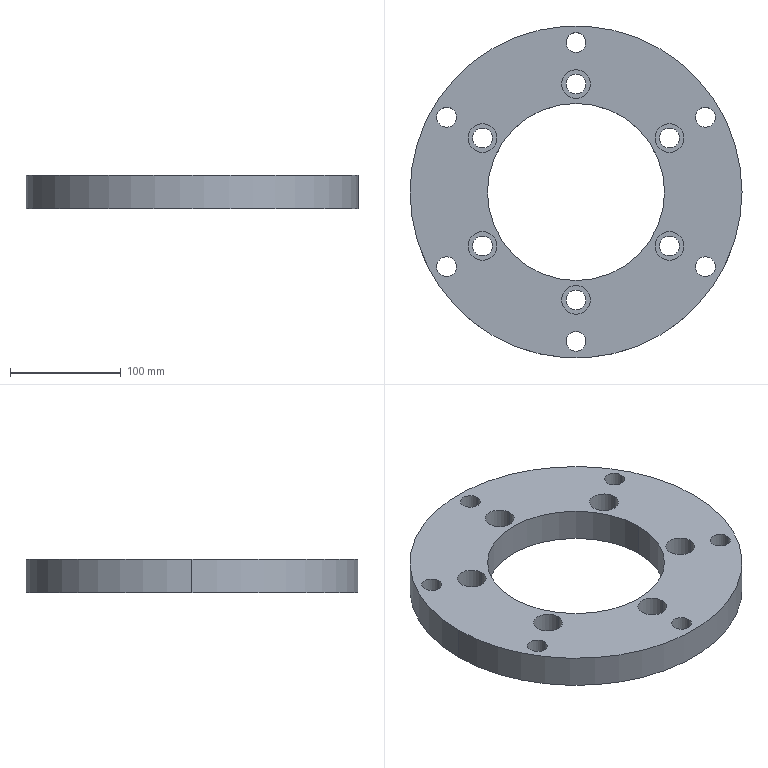Part | SolidWorks | features ICE 3, Extrusion 1 | 1 solid | 48 faces | box 300 x 300 x 30 mm | volume 1392605 mm3 | cylinder 40 | plane 8 | commonest cylinder face diameters 18 x24 26 x12 160 x2 300 x2
STEP:
#1=CARTESIAN_POINT('',(71.437,48.75,10.));
#2=VERTEX_POINT('',#1);
#3=CARTESIAN_POINT('',(97.437,48.75,10.));
#4=VERTEX_POINT('',#3);
#5=CARTESIAN_POINT('',(84.437,48.75,10.));
#6=DIRECTION('',(0.,0.,1.));
#7=DIRECTION('',(1.,0.,0.));
#8=AXIS2_PLACEMENT_3D('',#5,#6,#7);
#9=CIRCLE('',#8,13.);
#10=EDGE_CURVE('',#2,#4,#9,.T.);
#11=ORIENTED_EDGE('',*,*,#10,.F.);
#12=CARTESIAN_POINT('',(71.437,48.75,30.));
#13=VERTEX_POINT('',#12);
#14=CARTESIAN_POINT('',(71.437,48.75,10.));
#15=DIRECTION('',(0.,0.,1.));
#16=VECTOR('',#15,1000.);
#17=LINE('',#14,#16);
#18=EDGE_CURVE('',#2,#13,#17,.T.);
#19=ORIENTED_EDGE('',*,*,#18,.T.);
#20=CARTESIAN_POINT('',(97.437,48.75,30.));
#21=VERTEX_POINT('',#20);
#22=CARTESIAN_POINT('',(84.437,48.75,30.));
#23=DIRECTION('',(0.,0.,1.));
#24=DIRECTION('',(1.,0.,0.));
#25=AXIS2_PLACEMENT_3D('',#22,#23,#24);
#26=CIRCLE('',#25,13.);
#27=EDGE_CURVE('',#13,#21,#26,.T.);
#28=ORIENTED_EDGE('',*,*,#27,.T.);
#29=CARTESIAN_POINT('',(97.437,48.75,10.));
#30=DIRECTION('',(0.,0.,1.));
#31=VECTOR('',#30,1000.);
#32=LINE('',#29,#31);
#33=EDGE_CURVE('',#4,#21,#32,.T.);
#34=ORIENTED_EDGE('',*,*,#33,.F.);
#35=EDGE_LOOP('',(#11,#19,#28,#34));
#36=FACE_OUTER_BOUND('',#35,.T.);
#37=CARTESIAN_POINT('',(84.437,48.75,10.));
#38=DIRECTION('',(0.,0.,1.));
#39=DIRECTION('',(1.,0.,0.));
#40=AXIS2_PLACEMENT_3D('',#37,#38,#39);
#41=CYLINDRICAL_SURFACE('',#40,13.);
#42=ADVANCED_FACE('',(#36),#41,.F.);
#43=CARTESIAN_POINT('',(71.437,-48.75,10.));
#44=VERTEX_POINT('',#43);
#45=CARTESIAN_POINT('',(97.437,-48.75,10.));
#46=VERTEX_POINT('',#45);
#47=CARTESIAN_POINT('',(84.437,-48.75,10.));
#48=DIRECTION('',(0.,0.,1.));
#49=DIRECTION('',(1.,0.,0.));
#50=AXIS2_PLACEMENT_3D('',#47,#48,#49);
#51=CIRCLE('',#50,13.);
#52=EDGE_CURVE('',#44,#46,#51,.T.);
#53=ORIENTED_EDGE('',*,*,#52,.F.);
#54=CARTESIAN_POINT('',(71.437,-48.75,30.));
#55=VERTEX_POINT('',#54);
#56=CARTESIAN_POINT('',(71.437,-48.75,10.));
#57=DIRECTION('',(0.,0.,1.));
#58=VECTOR('',#57,1000.);
#59=LINE('',#56,#58);
#60=EDGE_CURVE('',#44,#55,#59,.T.);
#61=ORIENTED_EDGE('',*,*,#60,.T.);
#62=CARTESIAN_POINT('',(97.437,-48.75,30.));
#63=VERTEX_POINT('',#62);
#64=CARTESIAN_POINT('',(84.437,-48.75,30.));
#65=DIRECTION('',(0.,0.,1.));
#66=DIRECTION('',(1.,0.,0.));
#67=AXIS2_PLACEMENT_3D('',#64,#65,#66);
#68=CIRCLE('',#67,13.);
#69=EDGE_CURVE('',#55,#63,#68,.T.);
#70=ORIENTED_EDGE('',*,*,#69,.T.);
#71=CARTESIAN_POINT('',(97.437,-48.75,10.));
#72=DIRECTION('',(0.,0.,1.));
#73=VECTOR('',#72,1000.);
#74=LINE('',#71,#73);
#75=EDGE_CURVE('',#46,#63,#74,.T.);
#76=ORIENTED_EDGE('',*,*,#75,.F.);
#77=EDGE_LOOP('',(#53,#61,#70,#76));
#78=FACE_OUTER_BOUND('',#77,.T.);
#79=CARTESIAN_POINT('',(84.437,-48.75,10.));
#80=DIRECTION('',(0.,0.,1.));
#81=DIRECTION('',(1.,0.,0.));
#82=AXIS2_PLACEMENT_3D('',#79,#80,#81);
#83=CYLINDRICAL_SURFACE('',#82,13.);
#84=ADVANCED_FACE('',(#78),#83,.F.);
#85=CARTESIAN_POINT('',(-13.,-97.5,10.));
#86=VERTEX_POINT('',#85);
#87=CARTESIAN_POINT('',(13.,-97.5,10.));
#88=VERTEX_POINT('',#87);
#89=CARTESIAN_POINT('',(0.,-97.5,10.));
#90=DIRECTION('',(0.,0.,1.));
#91=DIRECTION('',(1.,0.,0.));
#92=AXIS2_PLACEMENT_3D('',#89,#90,#91);
#93=CIRCLE('',#92,13.);
#94=EDGE_CURVE('',#86,#88,#93,.T.);
#95=ORIENTED_EDGE('',*,*,#94,.F.);
#96=CARTESIAN_POINT('',(-13.,-97.5,30.));
#97=VERTEX_POINT('',#96);
#98=CARTESIAN_POINT('',(-13.,-97.5,10.));
#99=DIRECTION('',(0.,0.,1.));
#100=VECTOR('',#99,1000.);
#101=LINE('',#98,#100);
#102=EDGE_CURVE('',#86,#97,#101,.T.);
#103=ORIENTED_EDGE('',*,*,#102,.T.);
#104=CARTESIAN_POINT('',(13.,-97.5,30.));
#105=VERTEX_POINT('',#104);
#106=CARTESIAN_POINT('',(0.,-97.5,30.));
#107=DIRECTION('',(0.,0.,1.));
#108=DIRECTION('',(1.,0.,0.));
#109=AXIS2_PLACEMENT_3D('',#106,#107,#108);
#110=CIRCLE('',#109,13.);
#111=EDGE_CURVE('',#97,#105,#110,.T.);
#112=ORIENTED_EDGE('',*,*,#111,.T.);
#113=CARTESIAN_POINT('',(13.,-97.5,10.));
#114=DIRECTION('',(0.,0.,1.));
#115=VECTOR('',#114,1000.);
#116=LINE('',#113,#115);
#117=EDGE_CURVE('',#88,#105,#116,.T.);
#118=ORIENTED_EDGE('',*,*,#117,.F.);
#119=EDGE_LOOP('',(#95,#103,#112,#118));
#120=FACE_OUTER_BOUND('',#119,.T.);
#121=CARTESIAN_POINT('',(0.,-97.5,10.));
#122=DIRECTION('',(0.,0.,1.));
#123=DIRECTION('',(1.,0.,0.));
#124=AXIS2_PLACEMENT_3D('',#121,#122,#123);
#125=CYLINDRICAL_SURFACE('',#124,13.);
#126=ADVANCED_FACE('',(#120),#125,.F.);
#127=CARTESIAN_POINT('',(-97.437,-48.75,10.));
#128=VERTEX_POINT('',#127);
#129=CARTESIAN_POINT('',(-71.437,-48.75,10.));
#130=VERTEX_POINT('',#129);
#131=CARTESIAN_POINT('',(-84.437,-48.75,10.));
#132=DIRECTION('',(0.,0.,1.));
#133=DIRECTION('',(1.,0.,0.));
#134=AXIS2_PLACEMENT_3D('',#131,#132,#133);
#135=CIRCLE('',#134,13.);
#136=EDGE_CURVE('',#128,#130,#135,.T.);
#137=ORIENTED_EDGE('',*,*,#136,.F.);
#138=CARTESIAN_POINT('',(-97.437,-48.75,30.));
#139=VERTEX_POINT('',#138);
#140=CARTESIAN_POINT('',(-97.437,-48.75,10.));
#141=DIRECTION('',(0.,0.,1.));
#142=VECTOR('',#141,1000.);
#143=LINE('',#140,#142);
#144=EDGE_CURVE('',#128,#139,#143,.T.);
#145=ORIENTED_EDGE('',*,*,#144,.T.);
#146=CARTESIAN_POINT('',(-71.437,-48.75,30.));
#147=VERTEX_POINT('',#146);
#148=CARTESIAN_POINT('',(-84.437,-48.75,30.));
#149=DIRECTION('',(0.,0.,1.));
#150=DIRECTION('',(1.,0.,0.));
#151=AXIS2_PLACEMENT_3D('',#148,#149,#150);
#152=CIRCLE('',#151,13.);
#153=EDGE_CURVE('',#139,#147,#152,.T.);
#154=ORIENTED_EDGE('',*,*,#153,.T.);
#155=CARTESIAN_POINT('',(-71.437,-48.75,10.));
#156=DIRECTION('',(0.,0.,1.));
#157=VECTOR('',#156,1000.);
#158=LINE('',#155,#157);
#159=EDGE_CURVE('',#130,#147,#158,.T.);
#160=ORIENTED_EDGE('',*,*,#159,.F.);
#161=EDGE_LOOP('',(#137,#145,#154,#160));
#162=FACE_OUTER_BOUND('',#161,.T.);
#163=CARTESIAN_POINT('',(-84.437,-48.75,10.));
#164=DIRECTION('',(0.,0.,1.));
#165=DIRECTION('',(1.,0.,0.));
#166=AXIS2_PLACEMENT_3D('',#163,#164,#165);
#167=CYLINDRICAL_SURFACE('',#166,13.);
#168=ADVANCED_FACE('',(#162),#167,.F.);
#169=CARTESIAN_POINT('',(-97.437,48.75,10.));
#170=VERTEX_POINT('',#169);
#171=CARTESIAN_POINT('',(-71.437,48.75,10.));
#172=VERTEX_POINT('',#171);
#173=CARTESIAN_POINT('',(-84.437,48.75,10.));
#174=DIRECTION('',(0.,0.,1.));
#175=DIRECTION('',(1.,0.,0.));
#176=AXIS2_PLACEMENT_3D('',#173,#174,#175);
#177=CIRCLE('',#176,13.);
#178=EDGE_CURVE('',#170,#172,#177,.T.);
#179=ORIENTED_EDGE('',*,*,#178,.F.);
#180=CARTESIAN_POINT('',(-97.437,48.75,30.));
#181=VERTEX_POINT('',#180);
#182=CARTESIAN_POINT('',(-97.437,48.75,10.));
#183=DIRECTION('',(0.,0.,1.));
#184=VECTOR('',#183,1000.);
#185=LINE('',#182,#184);
#186=EDGE_CURVE('',#170,#181,#185,.T.);
#187=ORIENTED_EDGE('',*,*,#186,.T.);
#188=CARTESIAN_POINT('',(-71.437,48.75,30.));
#189=VERTEX_POINT('',#188);
#190=CARTESIAN_POINT('',(-84.437,48.75,30.));
#191=DIRECTION('',(0.,0.,1.));
#192=DIRECTION('',(1.,0.,0.));
#193=AXIS2_PLACEMENT_3D('',#190,#191,#192);
#194=CIRCLE('',#193,13.);
#195=EDGE_CURVE('',#181,#189,#194,.T.);
#196=ORIENTED_EDGE('',*,*,#195,.T.);
#197=CARTESIAN_POINT('',(-71.437,48.75,10.));
#198=DIRECTION('',(0.,0.,1.));
#199=VECTOR('',#198,1000.);
#200=LINE('',#197,#199);
#201=EDGE_CURVE('',#172,#189,#200,.T.);
#202=ORIENTED_EDGE('',*,*,#201,.F.);
#203=EDGE_LOOP('',(#179,#187,#196,#202));
#204=FACE_OUTER_BOUND('',#203,.T.);
#205=CARTESIAN_POINT('',(-84.437,48.75,10.));
#206=DIRECTION('',(0.,0.,1.));
#207=DIRECTION('',(1.,0.,0.));
#208=AXIS2_PLACEMENT_3D('',#205,#206,#207);
#209=CYLINDRICAL_SURFACE('',#208,13.);
#210=ADVANCED_FACE('',(#204),#209,.F.);
#211=CARTESIAN_POINT('',(-13.,97.5,10.));
#212=VERTEX_POINT('',#211);
#213=CARTESIAN_POINT('',(13.,97.5,10.));
#214=VERTEX_POINT('',#213);
#215=CARTESIAN_POINT('',(0.,97.5,10.));
#216=DIRECTION('',(0.,0.,1.));
#217=DIRECTION('',(1.,0.,0.));
#218=AXIS2_PLACEMENT_3D('',#215,#216,#217);
#219=CIRCLE('',#218,13.);
#220=EDGE_CURVE('',#212,#214,#219,.T.);
#221=ORIENTED_EDGE('',*,*,#220,.F.);
#222=CARTESIAN_POINT('',(-13.,97.5,30.));
#223=VERTEX_POINT('',#222);
#224=CARTESIAN_POINT('',(-13.,97.5,10.));
#225=DIRECTION('',(0.,0.,1.));
#226=VECTOR('',#225,1000.);
#227=LINE('',#224,#226);
#228=EDGE_CURVE('',#212,#223,#227,.T.);
#229=ORIENTED_EDGE('',*,*,#228,.T.);
#230=CARTESIAN_POINT('',(13.,97.5,30.));
#231=VERTEX_POINT('',#230);
#232=CARTESIAN_POINT('',(0.,97.5,30.));
#233=DIRECTION('',(0.,0.,1.));
#234=DIRECTION('',(1.,0.,0.));
#235=AXIS2_PLACEMENT_3D('',#232,#233,#234);
#236=CIRCLE('',#235,13.);
#237=EDGE_CURVE('',#223,#231,#236,.T.);
#238=ORIENTED_EDGE('',*,*,#237,.T.);
#239=CARTESIAN_POINT('',(13.,97.5,10.));
#240=DIRECTION('',(0.,0.,1.));
#241=VECTOR('',#240,1000.);
#242=LINE('',#239,#241);
#243=EDGE_CURVE('',#214,#231,#242,.T.);
#244=ORIENTED_EDGE('',*,*,#243,.F.);
#245=EDGE_LOOP('',(#221,#229,#238,#244));
#246=FACE_OUTER_BOUND('',#245,.T.);
#247=CARTESIAN_POINT('',(0.,97.5,10.));
#248=DIRECTION('',(0.,0.,1.));
#249=DIRECTION('',(1.,0.,0.));
#250=AXIS2_PLACEMENT_3D('',#247,#248,#249);
#251=CYLINDRICAL_SURFACE('',#250,13.);
#252=ADVANCED_FACE('',(#246),#251,.F.);
#253=CARTESIAN_POINT('',(-9.,135.,0.));
#254=VERTEX_POINT('',#253);
#255=CARTESIAN_POINT('',(9.,135.,0.));
#256=VERTEX_POINT('',#255);
#257=CARTESIAN_POINT('',(0.,135.,0.));
#258=DIRECTION('',(0.,0.,1.));
#259=DIRECTION('',(1.,0.,0.));
#260=AXIS2_PLACEMENT_3D('',#257,#258,#259);
#261=CIRCLE('',#260,9.);
#262=EDGE_CURVE('',#254,#256,#261,.T.);
#263=ORIENTED_EDGE('',*,*,#262,.F.);
#264=CARTESIAN_POINT('',(-9.,135.,30.));
#265=VERTEX_POINT('',#264);
#266=CARTESIAN_POINT('',(-9.,135.,0.));
#267=DIRECTION('',(0.,0.,1.));
#268=VECTOR('',#267,1000.);
#269=LINE('',#266,#268);
#270=EDGE_CURVE('',#254,#265,#269,.T.);
#271=ORIENTED_EDGE('',*,*,#270,.T.);
#272=CARTESIAN_POINT('',(9.,135.,30.));
#273=VERTEX_POINT('',#272);
#274=CARTESIAN_POINT('',(0.,135.,30.));
#275=DIRECTION('',(0.,0.,1.));
#276=DIRECTION('',(1.,0.,0.));
#277=AXIS2_PLACEMENT_3D('',#274,#275,#276);
#278=CIRCLE('',#277,9.);
#279=EDGE_CURVE('',#265,#273,#278,.T.);
#280=ORIENTED_EDGE('',*,*,#279,.T.);
#281=CARTESIAN_POINT('',(9.,135.,0.));
#282=DIRECTION('',(0.,0.,1.));
#283=VECTOR('',#282,1000.);
#284=LINE('',#281,#283);
#285=EDGE_CURVE('',#256,#273,#284,.T.);
#286=ORIENTED_EDGE('',*,*,#285,.F.);
#287=EDGE_LOOP('',(#263,#271,#280,#286));
#288=FACE_OUTER_BOUND('',#287,.T.);
#289=CARTESIAN_POINT('',(0.,135.,0.));
#290=DIRECTION('',(0.,0.,1.));
#291=DIRECTION('',(1.,0.,0.));
#292=AXIS2_PLACEMENT_3D('',#289,#290,#291);
#293=CYLINDRICAL_SURFACE('',#292,9.);
#294=ADVANCED_FACE('',(#288),#293,.F.);
#295=CARTESIAN_POINT('',(-125.913,67.5,0.));
#296=VERTEX_POINT('',#295);
#297=CARTESIAN_POINT('',(-107.913,67.5,0.));
#298=VERTEX_POINT('',#297);
#299=CARTESIAN_POINT('',(-116.913,67.5,0.));
#300=DIRECTION('',(0.,0.,1.));
#301=DIRECTION('',(1.,0.,0.));
#302=AXIS2_PLACEMENT_3D('',#299,#300,#301);
#303=CIRCLE('',#302,9.);
#304=EDGE_CURVE('',#296,#298,#303,.T.);
#305=ORIENTED_EDGE('',*,*,#304,.F.);
#306=CARTESIAN_POINT('',(-125.913,67.5,30.));
#307=VERTEX_POINT('',#306);
#308=CARTESIAN_POINT('',(-125.913,67.5,0.));
#309=DIRECTION('',(0.,0.,1.));
#310=VECTOR('',#309,1000.);
#311=LINE('',#308,#310);
#312=EDGE_CURVE('',#296,#307,#311,.T.);
#313=ORIENTED_EDGE('',*,*,#312,.T.);
#314=CARTESIAN_POINT('',(-107.913,67.5,30.));
#315=VERTEX_POINT('',#314);
#316=CARTESIAN_POINT('',(-116.913,67.5,30.));
#317=DIRECTION('',(0.,0.,1.));
#318=DIRECTION('',(1.,0.,0.));
#319=AXIS2_PLACEMENT_3D('',#316,#317,#318);
#320=CIRCLE('',#319,9.);
#321=EDGE_CURVE('',#307,#315,#320,.T.);
#322=ORIENTED_EDGE('',*,*,#321,.T.);
#323=CARTESIAN_POINT('',(-107.913,67.5,0.));
#324=DIRECTION('',(0.,0.,1.));
#325=VECTOR('',#324,1000.);
#326=LINE('',#323,#325);
#327=EDGE_CURVE('',#298,#315,#326,.T.);
#328=ORIENTED_EDGE('',*,*,#327,.F.);
#329=EDGE_LOOP('',(#305,#313,#322,#328));
#330=FACE_OUTER_BOUND('',#329,.T.);
#331=CARTESIAN_POINT('',(-116.913,67.5,0.));
#332=DIRECTION('',(0.,0.,1.));
#333=DIRECTION('',(1.,0.,0.));
#334=AXIS2_PLACEMENT_3D('',#331,#332,#333);
#335=CYLINDRICAL_SURFACE('',#334,9.);
#336=ADVANCED_FACE('',(#330),#335,.F.);
#337=CARTESIAN_POINT('',(-125.913,-67.5,0.));
#338=VERTEX_POINT('',#337);
#339=CARTESIAN_POINT('',(-107.913,-67.5,0.));
#340=VERTEX_POINT('',#339);
#341=CARTESIAN_POINT('',(-116.913,-67.5,0.));
#342=DIRECTION('',(0.,0.,1.));
#343=DIRECTION('',(1.,0.,0.));
#344=AXIS2_PLACEMENT_3D('',#341,#342,#343);
#345=CIRCLE('',#344,9.);
#346=EDGE_CURVE('',#338,#340,#345,.T.);
#347=ORIENTED_EDGE('',*,*,#346,.F.);
#348=CARTESIAN_POINT('',(-125.913,-67.5,30.));
#349=VERTEX_POINT('',#348);
#350=CARTESIAN_POINT('',(-125.913,-67.5,0.));
#351=DIRECTION('',(0.,0.,1.));
#352=VECTOR('',#351,1000.);
#353=LINE('',#350,#352);
#354=EDGE_CURVE('',#338,#349,#353,.T.);
#355=ORIENTED_EDGE('',*,*,#354,.T.);
#356=CARTESIAN_POINT('',(-107.913,-67.5,30.));
#357=VERTEX_POINT('',#356);
#358=CARTESIAN_POINT('',(-116.913,-67.5,30.));
#359=DIRECTION('',(0.,0.,1.));
#360=DIRECTION('',(1.,0.,0.));
#361=AXIS2_PLACEMENT_3D('',#358,#359,#360);
#362=CIRCLE('',#361,9.);
#363=EDGE_CURVE('',#349,#357,#362,.T.);
#364=ORIENTED_EDGE('',*,*,#363,.T.);
#365=CARTESIAN_POINT('',(-107.913,-67.5,0.));
#366=DIRECTION('',(0.,0.,1.));
#367=VECTOR('',#366,1000.);
#368=LINE('',#365,#367);
#369=EDGE_CURVE('',#340,#357,#368,.T.);
#370=ORIENTED_EDGE('',*,*,#369,.F.);
#371=EDGE_LOOP('',(#347,#355,#364,#370));
#372=FACE_OUTER_BOUND('',#371,.T.);
#373=CARTESIAN_POINT('',(-116.913,-67.5,0.));
#374=DIRECTION('',(0.,0.,1.));
#375=DIRECTION('',(1.,0.,0.));
#376=AXIS2_PLACEMENT_3D('',#373,#374,#375);
#377=CYLINDRICAL_SURFACE('',#376,9.);
#378=ADVANCED_FACE('',(#372),#377,.F.);
#379=CARTESIAN_POINT('',(-9.,-135.,0.));
#380=VERTEX_POINT('',#379);
#381=CARTESIAN_POINT('',(9.,-135.,0.));
#382=VERTEX_POINT('',#381);
#383=CARTESIAN_POINT('',(0.,-135.,0.));
#384=DIRECTION('',(0.,0.,1.));
#385=DIRECTION('',(1.,0.,0.));
#386=AXIS2_PLACEMENT_3D('',#383,#384,#385);
#387=CIRCLE('',#386,9.);
#388=EDGE_CURVE('',#380,#382,#387,.T.);
#389=ORIENTED_EDGE('',*,*,#388,.F.);
#390=CARTESIAN_POINT('',(-9.,-135.,30.));
#391=VERTEX_POINT('',#390);
#392=CARTESIAN_POINT('',(-9.,-135.,0.));
#393=DIRECTION('',(0.,0.,1.));
#394=VECTOR('',#393,1000.);
#395=LINE('',#392,#394);
#396=EDGE_CURVE('',#380,#391,#395,.T.);
#397=ORIENTED_EDGE('',*,*,#396,.T.);
#398=CARTESIAN_POINT('',(9.,-135.,30.));
#399=VERTEX_POINT('',#398);
#400=CARTESIAN_POINT('',(0.,-135.,30.));
#401=DIRECTION('',(0.,0.,1.));
#402=DIRECTION('',(1.,0.,0.));
#403=AXIS2_PLACEMENT_3D('',#400,#401,#402);
#404=CIRCLE('',#403,9.);
#405=EDGE_CURVE('',#391,#399,#404,.T.);
#406=ORIENTED_EDGE('',*,*,#405,.T.);
#407=CARTESIAN_POINT('',(9.,-135.,0.));
#408=DIRECTION('',(0.,0.,1.));
#409=VECTOR('',#408,1000.);
#410=LINE('',#407,#409);
#411=EDGE_CURVE('',#382,#399,#410,.T.);
#412=ORIENTED_EDGE('',*,*,#411,.F.);
#413=EDGE_LOOP('',(#389,#397,#406,#412));
#414=FACE_OUTER_BOUND('',#413,.T.);
#415=CARTESIAN_POINT('',(0.,-135.,0.));
#416=DIRECTION('',(0.,0.,1.));
#417=DIRECTION('',(1.,0.,0.));
#418=AXIS2_PLACEMENT_3D('',#415,#416,#417);
#419=CYLINDRICAL_SURFACE('',#418,9.);
#420=ADVANCED_FACE('',(#414),#419,.F.);
#421=CARTESIAN_POINT('',(107.913,-67.5,0.));
#422=VERTEX_POINT('',#421);
#423=CARTESIAN_POINT('',(125.913,-67.5,0.));
#424=VERTEX_POINT('',#423);
#425=CARTESIAN_POINT('',(116.913,-67.5,0.));
#426=DIRECTION('',(0.,0.,1.));
#427=DIRECTION('',(1.,0.,0.));
#428=AXIS2_PLACEMENT_3D('',#425,#426,#427);
#429=CIRCLE('',#428,9.);
#430=EDGE_CURVE('',#422,#424,#429,.T.);
#431=ORIENTED_EDGE('',*,*,#430,.F.);
#432=CARTESIAN_POINT('',(107.913,-67.5,30.));
#433=VERTEX_POINT('',#432);
#434=CARTESIAN_POINT('',(107.913,-67.5,0.));
#435=DIRECTION('',(0.,0.,1.));
#436=VECTOR('',#435,1000.);
#437=LINE('',#434,#436);
#438=EDGE_CURVE('',#422,#433,#437,.T.);
#439=ORIENTED_EDGE('',*,*,#438,.T.);
#440=CARTESIAN_POINT('',(125.913,-67.5,30.));
#441=VERTEX_POINT('',#440);
#442=CARTESIAN_POINT('',(116.913,-67.5,30.));
#443=DIRECTION('',(0.,0.,1.));
#444=DIRECTION('',(1.,0.,0.));
#445=AXIS2_PLACEMENT_3D('',#442,#443,#444);
#446=CIRCLE('',#445,9.);
#447=EDGE_CURVE('',#433,#441,#446,.T.);
#448=ORIENTED_EDGE('',*,*,#447,.T.);
#449=CARTESIAN_POINT('',(125.913,-67.5,0.));
#450=DIRECTION('',(0.,0.,1.));
#451=VECTOR('',#450,1000.);
#452=LINE('',#449,#451);
#453=EDGE_CURVE('',#424,#441,#452,.T.);
#454=ORIENTED_EDGE('',*,*,#453,.F.);
#455=EDGE_LOOP('',(#431,#439,#448,#454));
#456=FACE_OUTER_BOUND('',#455,.T.);
#457=CARTESIAN_POINT('',(116.913,-67.5,0.));
#458=DIRECTION('',(0.,0.,1.));
#459=DIRECTION('',(1.,0.,0.));
#460=AXIS2_PLACEMENT_3D('',#457,#458,#459);
#461=CYLINDRICAL_SURFACE('',#460,9.);
#462=ADVANCED_FACE('',(#456),#461,.F.);
#463=CARTESIAN_POINT('',(107.913,67.5,0.));
#464=VERTEX_POINT('',#463);
#465=CARTESIAN_POINT('',(125.913,67.5,0.));
#466=VERTEX_POINT('',#465);
#467=CARTESIAN_POINT('',(116.913,67.5,0.));
#468=DIRECTION('',(0.,0.,1.));
#469=DIRECTION('',(1.,0.,0.));
#470=AXIS2_PLACEMENT_3D('',#467,#468,#469);
#471=CIRCLE('',#470,9.);
#472=EDGE_CURVE('',#464,#466,#471,.T.);
#473=ORIENTED_EDGE('',*,*,#472,.F.);
#474=CARTESIAN_POINT('',(107.913,67.5,30.));
#475=VERTEX_POINT('',#474);
#476=CARTESIAN_POINT('',(107.913,67.5,0.));
#477=DIRECTION('',(0.,0.,1.));
#478=VECTOR('',#477,1000.);
#479=LINE('',#476,#478);
#480=EDGE_CURVE('',#464,#475,#479,.T.);
#481=ORIENTED_EDGE('',*,*,#480,.T.);
#482=CARTESIAN_POINT('',(125.913,67.5,30.));
#483=VERTEX_POINT('',#482);
#484=CARTESIAN_POINT('',(116.913,67.5,30.));
#485=DIRECTION('',(0.,0.,1.));
#486=DIRECTION('',(1.,0.,0.));
#487=AXIS2_PLACEMENT_3D('',#484,#485,#486);
#488=CIRCLE('',#487,9.);
#489=EDGE_CURVE('',#475,#483,#488,.T.);
#490=ORIENTED_EDGE('',*,*,#489,.T.);
#491=CARTESIAN_POINT('',(125.913,67.5,0.));
#492=DIRECTION('',(0.,0.,1.));
#493=VECTOR('',#492,1000.);
#494=LINE('',#491,#493);
#495=EDGE_CURVE('',#466,#483,#494,.T.);
#496=ORIENTED_EDGE('',*,*,#495,.F.);
#497=EDGE_LOOP('',(#473,#481,#490,#496));
#498=FACE_OUTER_BOUND('',#497,.T.);
#499=CARTESIAN_POINT('',(116.913,67.5,0.));
#500=DIRECTION('',(0.,0.,1.));
#501=DIRECTION('',(1.,0.,0.));
#502=AXIS2_PLACEMENT_3D('',#499,#500,#501);
#503=CYLINDRICAL_SURFACE('',#502,9.);
#504=ADVANCED_FACE('',(#498),#503,.F.);
#505=CARTESIAN_POINT('',(-80.,0.,30.));
#506=VERTEX_POINT('',#505);
#507=CARTESIAN_POINT('',(80.,0.,30.));
#508=VERTEX_POINT('',#507);
#509=CARTESIAN_POINT('',(0.,0.,30.));
#510=DIRECTION('',(0.,0.,1.));
#511=DIRECTION('',(1.,0.,0.));
#512=AXIS2_PLACEMENT_3D('',#509,#510,#511);
#513=CIRCLE('',#512,80.);
#514=EDGE_CURVE('',#506,#508,#513,.T.);
#515=ORIENTED_EDGE('',*,*,#514,.T.);
#516=CARTESIAN_POINT('',(80.,0.,0.));
#517=VERTEX_POINT('',#516);
#518=CARTESIAN_POINT('',(80.,0.,30.));
#519=DIRECTION('',(0.,0.,-1.));
#520=VECTOR('',#519,1000.);
#521=LINE('',#518,#520);
#522=EDGE_CURVE('',#508,#517,#521,.T.);
#523=ORIENTED_EDGE('',*,*,#522,.T.);
#524=CARTESIAN_POINT('',(-80.,0.,0.));
#525=VERTEX_POINT('',#524);
#526=CARTESIAN_POINT('',(0.,0.,0.));
#527=DIRECTION('',(0.,0.,1.));
#528=DIRECTION('',(1.,0.,0.));
#529=AXIS2_PLACEMENT_3D('',#526,#527,#528);
#530=CIRCLE('',#529,80.);
#531=EDGE_CURVE('',#525,#517,#530,.T.);
#532=ORIENTED_EDGE('',*,*,#531,.F.);
#533=CARTESIAN_POINT('',(-80.,0.,30.));
#534=DIRECTION('',(0.,0.,-1.));
#535=VECTOR('',#534,1000.);
#536=LINE('',#533,#535);
#537=EDGE_CURVE('',#506,#525,#536,.T.);
#538=ORIENTED_EDGE('',*,*,#537,.F.);
#539=EDGE_LOOP('',(#515,#523,#532,#538));
#540=FACE_OUTER_BOUND('',#539,.T.);
#541=CARTESIAN_POINT('',(0.,0.,30.));
#542=DIRECTION('',(0.,0.,-1.));
#543=DIRECTION('',(-1.,0.,0.));
#544=AXIS2_PLACEMENT_3D('',#541,#542,#543);
#545=CYLINDRICAL_SURFACE('',#544,80.);
#546=ADVANCED_FACE('',(#540),#545,.F.);
#547=CARTESIAN_POINT('',(150.,0.,30.));
#548=VERTEX_POINT('',#547);
#549=CARTESIAN_POINT('',(-150.,0.,30.));
#550=VERTEX_POINT('',#549);
#551=CARTESIAN_POINT('',(0.,0.,30.));
#552=DIRECTION('',(0.,0.,1.));
#553=DIRECTION('',(1.,0.,0.));
#554=AXIS2_PLACEMENT_3D('',#551,#552,#553);
#555=CIRCLE('',#554,150.);
#556=EDGE_CURVE('',#548,#550,#555,.T.);
#557=ORIENTED_EDGE('',*,*,#556,.F.);
#558=CARTESIAN_POINT('',(150.,0.,0.));
#559=VERTEX_POINT('',#558);
#560=CARTESIAN_POINT('',(150.,0.,30.));
#561=DIRECTION('',(0.,0.,-1.));
#562=VECTOR('',#561,1000.);
#563=LINE('',#560,#562);
#564=EDGE_CURVE('',#548,#559,#563,.T.);
#565=ORIENTED_EDGE('',*,*,#564,.T.);
#566=CARTESIAN_POINT('',(-150.,0.,0.));
#567=VERTEX_POINT('',#566);
#568=CARTESIAN_POINT('',(0.,0.,0.));
#569=DIRECTION('',(0.,0.,1.));
#570=DIRECTION('',(1.,0.,0.));
#571=AXIS2_PLACEMENT_3D('',#568,#569,#570);
#572=CIRCLE('',#571,150.);
#573=EDGE_CURVE('',#559,#567,#572,.T.);
#574=ORIENTED_EDGE('',*,*,#573,.T.);
#575=CARTESIAN_POINT('',(-150.,0.,30.));
#576=DIRECTION('',(0.,0.,-1.));
#577=VECTOR('',#576,1000.);
#578=LINE('',#575,#577);
#579=EDGE_CURVE('',#550,#567,#578,.T.);
#580=ORIENTED_EDGE('',*,*,#579,.F.);
#581=EDGE_LOOP('',(#557,#565,#574,#580));
#582=FACE_OUTER_BOUND('',#581,.T.);
#583=CARTESIAN_POINT('',(0.,0.,30.));
#584=DIRECTION('',(0.,0.,-1.));
#585=DIRECTION('',(-1.,0.,0.));
#586=AXIS2_PLACEMENT_3D('',#583,#584,#585);
#587=CYLINDRICAL_SURFACE('',#586,150.);
#588=ADVANCED_FACE('',(#582),#587,.T.);
#589=CARTESIAN_POINT('',(-9.,97.5,0.));
#590=VERTEX_POINT('',#589);
#591=CARTESIAN_POINT('',(9.,97.5,0.));
#592=VERTEX_POINT('',#591);
#593=CARTESIAN_POINT('',(0.,97.5,0.));
#594=DIRECTION('',(0.,0.,1.));
#595=DIRECTION('',(1.,0.,0.));
#596=AXIS2_PLACEMENT_3D('',#593,#594,#595);
#597=CIRCLE('',#596,9.);
#598=EDGE_CURVE('',#590,#592,#597,.T.);
#599=ORIENTED_EDGE('',*,*,#598,.F.);
#600=CARTESIAN_POINT('',(-9.,97.5,10.));
#601=VERTEX_POINT('',#600);
#602=CARTESIAN_POINT('',(-9.,97.5,0.));
#603=DIRECTION('',(0.,0.,1.));
#604=VECTOR('',#603,1000.);
#605=LINE('',#602,#604);
#606=EDGE_CURVE('',#590,#601,#605,.T.);
#607=ORIENTED_EDGE('',*,*,#606,.T.);
#608=CARTESIAN_POINT('',(9.,97.5,10.));
#609=VERTEX_POINT('',#608);
#610=CARTESIAN_POINT('',(0.,97.5,10.));
#611=DIRECTION('',(0.,0.,-1.));
#612=DIRECTION('',(1.,0.,0.));
#613=AXIS2_PLACEMENT_3D('',#610,#611,#612);
#614=CIRCLE('',#613,9.);
#615=EDGE_CURVE('',#609,#601,#614,.T.);
#616=ORIENTED_EDGE('',*,*,#615,.F.);
#617=CARTESIAN_POINT('',(9.,97.5,0.));
#618=DIRECTION('',(0.,0.,1.));
#619=VECTOR('',#618,1000.);
#620=LINE('',#617,#619);
#621=EDGE_CURVE('',#592,#609,#620,.T.);
#622=ORIENTED_EDGE('',*,*,#621,.F.);
#623=EDGE_LOOP('',(#599,#607,#616,#622));
#624=FACE_OUTER_BOUND('',#623,.T.);
#625=CARTESIAN_POINT('',(0.,97.5,0.));
#626=DIRECTION('',(0.,0.,1.));
#627=DIRECTION('',(1.,0.,0.));
#628=AXIS2_PLACEMENT_3D('',#625,#626,#627);
#629=CYLINDRICAL_SURFACE('',#628,9.);
#630=ADVANCED_FACE('',(#624),#629,.F.);
#631=CARTESIAN_POINT('',(-93.437,48.75,0.));
#632=VERTEX_POINT('',#631);
#633=CARTESIAN_POINT('',(-75.437,48.75,0.));
#634=VERTEX_POINT('',#633);
#635=CARTESIAN_POINT('',(-84.437,48.75,0.));
#636=DIRECTION('',(0.,0.,1.));
#637=DIRECTION('',(1.,0.,0.));
#638=AXIS2_PLACEMENT_3D('',#635,#636,#637);
#639=CIRCLE('',#638,9.);
#640=EDGE_CURVE('',#632,#634,#639,.T.);
#641=ORIENTED_EDGE('',*,*,#640,.F.);
#642=CARTESIAN_POINT('',(-93.437,48.75,10.));
#643=VERTEX_POINT('',#642);
#644=CARTESIAN_POINT('',(-93.437,48.75,0.));
#645=DIRECTION('',(0.,0.,1.));
#646=VECTOR('',#645,1000.);
#647=LINE('',#644,#646);
#648=EDGE_CURVE('',#632,#643,#647,.T.);
#649=ORIENTED_EDGE('',*,*,#648,.T.);
#650=CARTESIAN_POINT('',(-75.437,48.75,10.));
#651=VERTEX_POINT('',#650);
#652=CARTESIAN_POINT('',(-84.437,48.75,10.));
#653=DIRECTION('',(0.,0.,-1.));
#654=DIRECTION('',(1.,0.,0.));
#655=AXIS2_PLACEMENT_3D('',#652,#653,#654);
#656=CIRCLE('',#655,9.);
#657=EDGE_CURVE('',#651,#643,#656,.T.);
#658=ORIENTED_EDGE('',*,*,#657,.F.);
#659=CARTESIAN_POINT('',(-75.437,48.75,0.));
#660=DIRECTION('',(0.,0.,1.));
#661=VECTOR('',#660,1000.);
#662=LINE('',#659,#661);
#663=EDGE_CURVE('',#634,#651,#662,.T.);
#664=ORIENTED_EDGE('',*,*,#663,.F.);
#665=EDGE_LOOP('',(#641,#649,#658,#664));
#666=FACE_OUTER_BOUND('',#665,.T.);
#667=CARTESIAN_POINT('',(-84.437,48.75,0.));
#668=DIRECTION('',(0.,0.,1.));
#669=DIRECTION('',(1.,0.,0.));
#670=AXIS2_PLACEMENT_3D('',#667,#668,#669);
#671=CYLINDRICAL_SURFACE('',#670,9.);
#672=ADVANCED_FACE('',(#666),#671,.F.);
#673=CARTESIAN_POINT('',(-93.437,-48.75,0.));
#674=VERTEX_POINT('',#673);
#675=CARTESIAN_POINT('',(-75.437,-48.75,0.));
#676=VERTEX_POINT('',#675);
#677=CARTESIAN_POINT('',(-84.437,-48.75,0.));
#678=DIRECTION('',(0.,0.,1.));
#679=DIRECTION('',(1.,0.,0.));
#680=AXIS2_PLACEMENT_3D('',#677,#678,#679);
#681=CIRCLE('',#680,9.);
#682=EDGE_CURVE('',#674,#676,#681,.T.);
#683=ORIENTED_EDGE('',*,*,#682,.F.);
#684=CARTESIAN_POINT('',(-93.437,-48.75,10.));
#685=VERTEX_POINT('',#684);
#686=CARTESIAN_POINT('',(-93.437,-48.75,0.));
#687=DIRECTION('',(0.,0.,1.));
#688=VECTOR('',#687,1000.);
#689=LINE('',#686,#688);
#690=EDGE_CURVE('',#674,#685,#689,.T.);
#691=ORIENTED_EDGE('',*,*,#690,.T.);
#692=CARTESIAN_POINT('',(-75.437,-48.75,10.));
#693=VERTEX_POINT('',#692);
#694=CARTESIAN_POINT('',(-84.437,-48.75,10.));
#695=DIRECTION('',(0.,0.,-1.));
#696=DIRECTION('',(1.,0.,0.));
#697=AXIS2_PLACEMENT_3D('',#694,#695,#696);
#698=CIRCLE('',#697,9.);
#699=EDGE_CURVE('',#693,#685,#698,.T.);
#700=ORIENTED_EDGE('',*,*,#699,.F.);
#701=CARTESIAN_POINT('',(-75.437,-48.75,0.));
#702=DIRECTION('',(0.,0.,1.));
#703=VECTOR('',#702,1000.);
#704=LINE('',#701,#703);
#705=EDGE_CURVE('',#676,#693,#704,.T.);
#706=ORIENTED_EDGE('',*,*,#705,.F.);
#707=EDGE_LOOP('',(#683,#691,#700,#706));
#708=FACE_OUTER_BOUND('',#707,.T.);
#709=CARTESIAN_POINT('',(-84.437,-48.75,0.));
#710=DIRECTION('',(0.,0.,1.));
#711=DIRECTION('',(1.,0.,0.));
#712=AXIS2_PLACEMENT_3D('',#709,#710,#711);
#713=CYLINDRICAL_SURFACE('',#712,9.);
#714=ADVANCED_FACE('',(#708),#713,.F.);
#715=CARTESIAN_POINT('',(-9.,-97.5,0.));
#716=VERTEX_POINT('',#715);
#717=CARTESIAN_POINT('',(9.,-97.5,0.));
#718=VERTEX_POINT('',#717);
#719=CARTESIAN_POINT('',(0.,-97.5,0.));
#720=DIRECTION('',(0.,0.,1.));
#721=DIRECTION('',(1.,0.,0.));
#722=AXIS2_PLACEMENT_3D('',#719,#720,#721);
#723=CIRCLE('',#722,9.);
#724=EDGE_CURVE('',#716,#718,#723,.T.);
#725=ORIENTED_EDGE('',*,*,#724,.F.);
#726=CARTESIAN_POINT('',(-9.,-97.5,10.));
#727=VERTEX_POINT('',#726);
#728=CARTESIAN_POINT('',(-9.,-97.5,0.));
#729=DIRECTION('',(0.,0.,1.));
#730=VECTOR('',#729,1000.);
#731=LINE('',#728,#730);
#732=EDGE_CURVE('',#716,#727,#731,.T.);
#733=ORIENTED_EDGE('',*,*,#732,.T.);
#734=CARTESIAN_POINT('',(9.,-97.5,10.));
#735=VERTEX_POINT('',#734);
#736=CARTESIAN_POINT('',(0.,-97.5,10.));
#737=DIRECTION('',(0.,0.,-1.));
#738=DIRECTION('',(1.,0.,0.));
#739=AXIS2_PLACEMENT_3D('',#736,#737,#738);
#740=CIRCLE('',#739,9.);
#741=EDGE_CURVE('',#735,#727,#740,.T.);
#742=ORIENTED_EDGE('',*,*,#741,.F.);
#743=CARTESIAN_POINT('',(9.,-97.5,0.));
#744=DIRECTION('',(0.,0.,1.));
#745=VECTOR('',#744,1000.);
#746=LINE('',#743,#745);
#747=EDGE_CURVE('',#718,#735,#746,.T.);
#748=ORIENTED_EDGE('',*,*,#747,.F.);
#749=EDGE_LOOP('',(#725,#733,#742,#748));
#750=FACE_OUTER_BOUND('',#749,.T.);
#751=CARTESIAN_POINT('',(0.,-97.5,0.));
#752=DIRECTION('',(0.,0.,1.));
#753=DIRECTION('',(1.,0.,0.));
#754=AXIS2_PLACEMENT_3D('',#751,#752,#753);
#755=CYLINDRICAL_SURFACE('',#754,9.);
#756=ADVANCED_FACE('',(#750),#755,.F.);
#757=CARTESIAN_POINT('',(75.437,-48.75,0.));
#758=VERTEX_POINT('',#757);
#759=CARTESIAN_POINT('',(93.437,-48.75,0.));
#760=VERTEX_POINT('',#759);
#761=CARTESIAN_POINT('',(84.437,-48.75,0.));
#762=DIRECTION('',(0.,0.,1.));
#763=DIRECTION('',(1.,0.,0.));
#764=AXIS2_PLACEMENT_3D('',#761,#762,#763);
#765=CIRCLE('',#764,9.);
#766=EDGE_CURVE('',#758,#760,#765,.T.);
#767=ORIENTED_EDGE('',*,*,#766,.F.);
#768=CARTESIAN_POINT('',(75.437,-48.75,10.));
#769=VERTEX_POINT('',#768);
#770=CARTESIAN_POINT('',(75.437,-48.75,0.));
#771=DIRECTION('',(0.,0.,1.));
#772=VECTOR('',#771,1000.);
#773=LINE('',#770,#772);
#774=EDGE_CURVE('',#758,#769,#773,.T.);
#775=ORIENTED_EDGE('',*,*,#774,.T.);
#776=CARTESIAN_POINT('',(93.437,-48.75,10.));
#777=VERTEX_POINT('',#776);
#778=CARTESIAN_POINT('',(84.437,-48.75,10.));
#779=DIRECTION('',(0.,0.,-1.));
#780=DIRECTION('',(1.,0.,0.));
#781=AXIS2_PLACEMENT_3D('',#778,#779,#780);
#782=CIRCLE('',#781,9.);
#783=EDGE_CURVE('',#777,#769,#782,.T.);
#784=ORIENTED_EDGE('',*,*,#783,.F.);
#785=CARTESIAN_POINT('',(93.437,-48.75,0.));
#786=DIRECTION('',(0.,0.,1.));
#787=VECTOR('',#786,1000.);
#788=LINE('',#785,#787);
#789=EDGE_CURVE('',#760,#777,#788,.T.);
#790=ORIENTED_EDGE('',*,*,#789,.F.);
#791=EDGE_LOOP('',(#767,#775,#784,#790));
#792=FACE_OUTER_BOUND('',#791,.T.);
#793=CARTESIAN_POINT('',(84.437,-48.75,0.));
#794=DIRECTION('',(0.,0.,1.));
#795=DIRECTION('',(1.,0.,0.));
#796=AXIS2_PLACEMENT_3D('',#793,#794,#795);
#797=CYLINDRICAL_SURFACE('',#796,9.);
#798=ADVANCED_FACE('',(#792),#797,.F.);
#799=CARTESIAN_POINT('',(75.437,48.75,0.));
#800=VERTEX_POINT('',#799);
#801=CARTESIAN_POINT('',(93.437,48.75,0.));
#802=VERTEX_POINT('',#801);
#803=CARTESIAN_POINT('',(84.437,48.75,0.));
#804=DIRECTION('',(0.,0.,1.));
#805=DIRECTION('',(1.,0.,0.));
#806=AXIS2_PLACEMENT_3D('',#803,#804,#805);
#807=CIRCLE('',#806,9.);
#808=EDGE_CURVE('',#800,#802,#807,.T.);
#809=ORIENTED_EDGE('',*,*,#808,.F.);
#810=CARTESIAN_POINT('',(75.437,48.75,10.));
#811=VERTEX_POINT('',#810);
#812=CARTESIAN_POINT('',(75.437,48.75,0.));
#813=DIRECTION('',(0.,0.,1.));
#814=VECTOR('',#813,1000.);
#815=LINE('',#812,#814);
#816=EDGE_CURVE('',#800,#811,#815,.T.);
#817=ORIENTED_EDGE('',*,*,#816,.T.);
#818=CARTESIAN_POINT('',(93.437,48.75,10.));
#819=VERTEX_POINT('',#818);
#820=CARTESIAN_POINT('',(84.437,48.75,10.));
#821=DIRECTION('',(0.,0.,-1.));
#822=DIRECTION('',(1.,0.,0.));
#823=AXIS2_PLACEMENT_3D('',#820,#821,#822);
#824=CIRCLE('',#823,9.);
#825=EDGE_CURVE('',#819,#811,#824,.T.);
#826=ORIENTED_EDGE('',*,*,#825,.F.);
#827=CARTESIAN_POINT('',(93.437,48.75,0.));
#828=DIRECTION('',(0.,0.,1.));
#829=VECTOR('',#828,1000.);
#830=LINE('',#827,#829);
#831=EDGE_CURVE('',#802,#819,#830,.T.);
#832=ORIENTED_EDGE('',*,*,#831,.F.);
#833=EDGE_LOOP('',(#809,#817,#826,#832));
#834=FACE_OUTER_BOUND('',#833,.T.);
#835=CARTESIAN_POINT('',(84.437,48.75,0.));
#836=DIRECTION('',(0.,0.,1.));
#837=DIRECTION('',(1.,0.,0.));
#838=AXIS2_PLACEMENT_3D('',#835,#836,#837);
#839=CYLINDRICAL_SURFACE('',#838,9.);
#840=ADVANCED_FACE('',(#834),#839,.F.);
#841=ORIENTED_EDGE('',*,*,#816,.F.);
#842=CARTESIAN_POINT('',(84.437,48.75,0.));
#843=DIRECTION('',(0.,0.,1.));
#844=DIRECTION('',(1.,0.,0.));
#845=AXIS2_PLACEMENT_3D('',#842,#843,#844);
#846=CIRCLE('',#845,9.);
#847=EDGE_CURVE('',#802,#800,#846,.T.);
#848=ORIENTED_EDGE('',*,*,#847,.F.);
#849=ORIENTED_EDGE('',*,*,#831,.T.);
#850=CARTESIAN_POINT('',(84.437,48.75,10.));
#851=DIRECTION('',(0.,0.,-1.));
#852=DIRECTION('',(1.,0.,0.));
#853=AXIS2_PLACEMENT_3D('',#850,#851,#852);
#854=CIRCLE('',#853,9.);
#855=EDGE_CURVE('',#811,#819,#854,.T.);
#856=ORIENTED_EDGE('',*,*,#855,.F.);
#857=EDGE_LOOP('',(#841,#848,#849,#856));
#858=FACE_OUTER_BOUND('',#857,.T.);
#859=CARTESIAN_POINT('',(84.437,48.75,0.));
#860=DIRECTION('',(0.,0.,1.));
#861=DIRECTION('',(1.,0.,0.));
#862=AXIS2_PLACEMENT_3D('',#859,#860,#861);
#863=CYLINDRICAL_SURFACE('',#862,9.);
#864=ADVANCED_FACE('',(#858),#863,.F.);
#865=ORIENTED_EDGE('',*,*,#774,.F.);
#866=CARTESIAN_POINT('',(84.437,-48.75,0.));
#867=DIRECTION('',(0.,0.,1.));
#868=DIRECTION('',(1.,0.,0.));
#869=AXIS2_PLACEMENT_3D('',#866,#867,#868);
#870=CIRCLE('',#869,9.);
#871=EDGE_CURVE('',#760,#758,#870,.T.);
#872=ORIENTED_EDGE('',*,*,#871,.F.);
#873=ORIENTED_EDGE('',*,*,#789,.T.);
#874=CARTESIAN_POINT('',(84.437,-48.75,10.));
#875=DIRECTION('',(0.,0.,-1.));
#876=DIRECTION('',(1.,0.,0.));
#877=AXIS2_PLACEMENT_3D('',#874,#875,#876);
#878=CIRCLE('',#877,9.);
#879=EDGE_CURVE('',#769,#777,#878,.T.);
#880=ORIENTED_EDGE('',*,*,#879,.F.);
#881=EDGE_LOOP('',(#865,#872,#873,#880));
#882=FACE_OUTER_BOUND('',#881,.T.);
#883=CARTESIAN_POINT('',(84.437,-48.75,0.));
#884=DIRECTION('',(0.,0.,1.));
#885=DIRECTION('',(1.,0.,0.));
#886=AXIS2_PLACEMENT_3D('',#883,#884,#885);
#887=CYLINDRICAL_SURFACE('',#886,9.);
#888=ADVANCED_FACE('',(#882),#887,.F.);
#889=ORIENTED_EDGE('',*,*,#732,.F.);
#890=CARTESIAN_POINT('',(0.,-97.5,0.));
#891=DIRECTION('',(0.,0.,1.));
#892=DIRECTION('',(1.,0.,0.));
#893=AXIS2_PLACEMENT_3D('',#890,#891,#892);
#894=CIRCLE('',#893,9.);
#895=EDGE_CURVE('',#718,#716,#894,.T.);
#896=ORIENTED_EDGE('',*,*,#895,.F.);
#897=ORIENTED_EDGE('',*,*,#747,.T.);
#898=CARTESIAN_POINT('',(0.,-97.5,10.));
#899=DIRECTION('',(0.,0.,-1.));
#900=DIRECTION('',(1.,0.,0.));
#901=AXIS2_PLACEMENT_3D('',#898,#899,#900);
#902=CIRCLE('',#901,9.);
#903=EDGE_CURVE('',#727,#735,#902,.T.);
#904=ORIENTED_EDGE('',*,*,#903,.F.);
#905=EDGE_LOOP('',(#889,#896,#897,#904));
#906=FACE_OUTER_BOUND('',#905,.T.);
#907=CARTESIAN_POINT('',(0.,-97.5,0.));
#908=DIRECTION('',(0.,0.,1.));
#909=DIRECTION('',(1.,0.,0.));
#910=AXIS2_PLACEMENT_3D('',#907,#908,#909);
#911=CYLINDRICAL_SURFACE('',#910,9.);
#912=ADVANCED_FACE('',(#906),#911,.F.);
#913=ORIENTED_EDGE('',*,*,#690,.F.);
#914=CARTESIAN_POINT('',(-84.437,-48.75,0.));
#915=DIRECTION('',(0.,0.,1.));
#916=DIRECTION('',(1.,0.,0.));
#917=AXIS2_PLACEMENT_3D('',#914,#915,#916);
#918=CIRCLE('',#917,9.);
#919=EDGE_CURVE('',#676,#674,#918,.T.);
#920=ORIENTED_EDGE('',*,*,#919,.F.);
#921=ORIENTED_EDGE('',*,*,#705,.T.);
#922=CARTESIAN_POINT('',(-84.437,-48.75,10.));
#923=DIRECTION('',(0.,0.,-1.));
#924=DIRECTION('',(1.,0.,0.));
#925=AXIS2_PLACEMENT_3D('',#922,#923,#924);
#926=CIRCLE('',#925,9.);
#927=EDGE_CURVE('',#685,#693,#926,.T.);
#928=ORIENTED_EDGE('',*,*,#927,.F.);
#929=EDGE_LOOP('',(#913,#920,#921,#928));
#930=FACE_OUTER_BOUND('',#929,.T.);
#931=CARTESIAN_POINT('',(-84.437,-48.75,0.));
#932=DIRECTION('',(0.,0.,1.));
#933=DIRECTION('',(1.,0.,0.));
#934=AXIS2_PLACEMENT_3D('',#931,#932,#933);
#935=CYLINDRICAL_SURFACE('',#934,9.);
#936=ADVANCED_FACE('',(#930),#935,.F.);
#937=ORIENTED_EDGE('',*,*,#648,.F.);
#938=CARTESIAN_POINT('',(-84.437,48.75,0.));
#939=DIRECTION('',(0.,0.,1.));
#940=DIRECTION('',(1.,0.,0.));
#941=AXIS2_PLACEMENT_3D('',#938,#939,#940);
#942=CIRCLE('',#941,9.);
#943=EDGE_CURVE('',#634,#632,#942,.T.);
#944=ORIENTED_EDGE('',*,*,#943,.F.);
#945=ORIENTED_EDGE('',*,*,#663,.T.);
#946=CARTESIAN_POINT('',(-84.437,48.75,10.));
#947=DIRECTION('',(0.,0.,-1.));
#948=DIRECTION('',(1.,0.,0.));
#949=AXIS2_PLACEMENT_3D('',#946,#947,#948);
#950=CIRCLE('',#949,9.);
#951=EDGE_CURVE('',#643,#651,#950,.T.);
#952=ORIENTED_EDGE('',*,*,#951,.F.);
#953=EDGE_LOOP('',(#937,#944,#945,#952));
#954=FACE_OUTER_BOUND('',#953,.T.);
#955=CARTESIAN_POINT('',(-84.437,48.75,0.));
#956=DIRECTION('',(0.,0.,1.));
#957=DIRECTION('',(1.,0.,0.));
#958=AXIS2_PLACEMENT_3D('',#955,#956,#957);
#959=CYLINDRICAL_SURFACE('',#958,9.);
#960=ADVANCED_FACE('',(#954),#959,.F.);
#961=ORIENTED_EDGE('',*,*,#606,.F.);
#962=CARTESIAN_POINT('',(0.,97.5,0.));
#963=DIRECTION('',(0.,0.,1.));
#964=DIRECTION('',(1.,0.,0.));
#965=AXIS2_PLACEMENT_3D('',#962,#963,#964);
#966=CIRCLE('',#965,9.);
#967=EDGE_CURVE('',#592,#590,#966,.T.);
#968=ORIENTED_EDGE('',*,*,#967,.F.);
#969=ORIENTED_EDGE('',*,*,#621,.T.);
#970=CARTESIAN_POINT('',(0.,97.5,10.));
#971=DIRECTION('',(0.,0.,-1.));
#972=DIRECTION('',(1.,0.,0.));
#973=AXIS2_PLACEMENT_3D('',#970,#971,#972);
#974=CIRCLE('',#973,9.);
#975=EDGE_CURVE('',#601,#609,#974,.T.);
#976=ORIENTED_EDGE('',*,*,#975,.F.);
#977=EDGE_LOOP('',(#961,#968,#969,#976));
#978=FACE_OUTER_BOUND('',#977,.T.);
#979=CARTESIAN_POINT('',(0.,97.5,0.));
#980=DIRECTION('',(0.,0.,1.));
#981=DIRECTION('',(1.,0.,0.));
#982=AXIS2_PLACEMENT_3D('',#979,#980,#981);
#983=CYLINDRICAL_SURFACE('',#982,9.);
#984=ADVANCED_FACE('',(#978),#983,.F.);
#985=CARTESIAN_POINT('',(0.,97.5,30.));
#986=DIRECTION('',(0.,0.,1.));
#987=DIRECTION('',(1.,0.,0.));
#988=AXIS2_PLACEMENT_3D('',#985,#986,#987);
#989=CIRCLE('',#988,13.);
#990=EDGE_CURVE('',#231,#223,#989,.T.);
#991=ORIENTED_EDGE('',*,*,#990,.F.);
#992=ORIENTED_EDGE('',*,*,#237,.F.);
#993=EDGE_LOOP('',(#991,#992));
#994=FACE_BOUND('',#993,.T.);
#995=CARTESIAN_POINT('',(-84.437,48.75,30.));
#996=DIRECTION('',(0.,0.,1.));
#997=DIRECTION('',(1.,0.,0.));
#998=AXIS2_PLACEMENT_3D('',#995,#996,#997);
#999=CIRCLE('',#998,13.);
#1000=EDGE_CURVE('',#189,#181,#999,.T.);
#1001=ORIENTED_EDGE('',*,*,#1000,.F.);
#1002=ORIENTED_EDGE('',*,*,#195,.F.);
#1003=EDGE_LOOP('',(#1001,#1002));
#1004=FACE_BOUND('',#1003,.T.);
#1005=CARTESIAN_POINT('',(-84.437,-48.75,30.));
#1006=DIRECTION('',(0.,0.,1.));
#1007=DIRECTION('',(1.,0.,0.));
#1008=AXIS2_PLACEMENT_3D('',#1005,#1006,#1007);
#1009=CIRCLE('',#1008,13.);
#1010=EDGE_CURVE('',#147,#139,#1009,.T.);
#1011=ORIENTED_EDGE('',*,*,#1010,.F.);
#1012=ORIENTED_EDGE('',*,*,#153,.F.);
#1013=EDGE_LOOP('',(#1011,#1012));
#1014=FACE_BOUND('',#1013,.T.);
#1015=CARTESIAN_POINT('',(0.,-97.5,30.));
#1016=DIRECTION('',(0.,0.,1.));
#1017=DIRECTION('',(1.,0.,0.));
#1018=AXIS2_PLACEMENT_3D('',#1015,#1016,#1017);
#1019=CIRCLE('',#1018,13.);
#1020=EDGE_CURVE('',#105,#97,#1019,.T.);
#1021=ORIENTED_EDGE('',*,*,#1020,.F.);
#1022=ORIENTED_EDGE('',*,*,#111,.F.);
#1023=EDGE_LOOP('',(#1021,#1022));
#1024=FACE_BOUND('',#1023,.T.);
#1025=CARTESIAN_POINT('',(84.437,-48.75,30.));
#1026=DIRECTION('',(0.,0.,1.));
#1027=DIRECTION('',(1.,0.,0.));
#1028=AXIS2_PLACEMENT_3D('',#1025,#1026,#1027);
#1029=CIRCLE('',#1028,13.);
#1030=EDGE_CURVE('',#63,#55,#1029,.T.);
#1031=ORIENTED_EDGE('',*,*,#1030,.F.);
#1032=ORIENTED_EDGE('',*,*,#69,.F.);
#1033=EDGE_LOOP('',(#1031,#1032));
#1034=FACE_BOUND('',#1033,.T.);
#1035=CARTESIAN_POINT('',(84.437,48.75,30.));
#1036=DIRECTION('',(0.,0.,1.));
#1037=DIRECTION('',(1.,0.,0.));
#1038=AXIS2_PLACEMENT_3D('',#1035,#1036,#1037);
#1039=CIRCLE('',#1038,13.);
#1040=EDGE_CURVE('',#21,#13,#1039,.T.);
#1041=ORIENTED_EDGE('',*,*,#1040,.F.);
#1042=ORIENTED_EDGE('',*,*,#27,.F.);
#1043=EDGE_LOOP('',(#1041,#1042));
#1044=FACE_BOUND('',#1043,.T.);
#1045=CARTESIAN_POINT('',(0.,135.,30.));
#1046=DIRECTION('',(0.,0.,1.));
#1047=DIRECTION('',(1.,0.,0.));
#1048=AXIS2_PLACEMENT_3D('',#1045,#1046,#1047);
#1049=CIRCLE('',#1048,9.);
#1050=EDGE_CURVE('',#273,#265,#1049,.T.);
#1051=ORIENTED_EDGE('',*,*,#1050,.F.);
#1052=ORIENTED_EDGE('',*,*,#279,.F.);
#1053=EDGE_LOOP('',(#1051,#1052));
#1054=FACE_BOUND('',#1053,.T.);
#1055=CARTESIAN_POINT('',(-116.913,67.5,30.));
#1056=DIRECTION('',(0.,0.,1.));
#1057=DIRECTION('',(1.,0.,0.));
#1058=AXIS2_PLACEMENT_3D('',#1055,#1056,#1057);
#1059=CIRCLE('',#1058,9.);
#1060=EDGE_CURVE('',#315,#307,#1059,.T.);
#1061=ORIENTED_EDGE('',*,*,#1060,.F.);
#1062=ORIENTED_EDGE('',*,*,#321,.F.);
#1063=EDGE_LOOP('',(#1061,#1062));
#1064=FACE_BOUND('',#1063,.T.);
#1065=CARTESIAN_POINT('',(-116.913,-67.5,30.));
#1066=DIRECTION('',(0.,0.,1.));
#1067=DIRECTION('',(1.,0.,0.));
#1068=AXIS2_PLACEMENT_3D('',#1065,#1066,#1067);
#1069=CIRCLE('',#1068,9.);
#1070=EDGE_CURVE('',#357,#349,#1069,.T.);
#1071=ORIENTED_EDGE('',*,*,#1070,.F.);
#1072=ORIENTED_EDGE('',*,*,#363,.F.);
#1073=EDGE_LOOP('',(#1071,#1072));
#1074=FACE_BOUND('',#1073,.T.);
#1075=CARTESIAN_POINT('',(0.,-135.,30.));
#1076=DIRECTION('',(0.,0.,1.));
#1077=DIRECTION('',(1.,0.,0.));
#1078=AXIS2_PLACEMENT_3D('',#1075,#1076,#1077);
#1079=CIRCLE('',#1078,9.);
#1080=EDGE_CURVE('',#399,#391,#1079,.T.);
#1081=ORIENTED_EDGE('',*,*,#1080,.F.);
#1082=ORIENTED_EDGE('',*,*,#405,.F.);
#1083=EDGE_LOOP('',(#1081,#1082));
#1084=FACE_BOUND('',#1083,.T.);
#1085=CARTESIAN_POINT('',(116.913,-67.5,30.));
#1086=DIRECTION('',(0.,0.,1.));
#1087=DIRECTION('',(1.,0.,0.));
#1088=AXIS2_PLACEMENT_3D('',#1085,#1086,#1087);
#1089=CIRCLE('',#1088,9.);
#1090=EDGE_CURVE('',#441,#433,#1089,.T.);
#1091=ORIENTED_EDGE('',*,*,#1090,.F.);
#1092=ORIENTED_EDGE('',*,*,#447,.F.);
#1093=EDGE_LOOP('',(#1091,#1092));
#1094=FACE_BOUND('',#1093,.T.);
#1095=CARTESIAN_POINT('',(116.913,67.5,30.));
#1096=DIRECTION('',(0.,0.,1.));
#1097=DIRECTION('',(1.,0.,0.));
#1098=AXIS2_PLACEMENT_3D('',#1095,#1096,#1097);
#1099=CIRCLE('',#1098,9.);
#1100=EDGE_CURVE('',#483,#475,#1099,.T.);
#1101=ORIENTED_EDGE('',*,*,#1100,.F.);
#1102=ORIENTED_EDGE('',*,*,#489,.F.);
#1103=EDGE_LOOP('',(#1101,#1102));
#1104=FACE_BOUND('',#1103,.T.);
#1105=CARTESIAN_POINT('',(0.,0.,30.));
#1106=DIRECTION('',(0.,0.,1.));
#1107=DIRECTION('',(1.,0.,0.));
#1108=AXIS2_PLACEMENT_3D('',#1105,#1106,#1107);
#1109=CIRCLE('',#1108,150.);
#1110=EDGE_CURVE('',#550,#548,#1109,.T.);
#1111=ORIENTED_EDGE('',*,*,#1110,.T.);
#1112=ORIENTED_EDGE('',*,*,#556,.T.);
#1113=EDGE_LOOP('',(#1111,#1112));
#1114=FACE_OUTER_BOUND('',#1113,.T.);
#1115=ORIENTED_EDGE('',*,*,#514,.F.);
#1116=CARTESIAN_POINT('',(0.,0.,30.));
#1117=DIRECTION('',(0.,0.,1.));
#1118=DIRECTION('',(1.,0.,0.));
#1119=AXIS2_PLACEMENT_3D('',#1116,#1117,#1118);
#1120=CIRCLE('',#1119,80.);
#1121=EDGE_CURVE('',#508,#506,#1120,.T.);
#1122=ORIENTED_EDGE('',*,*,#1121,.F.);
#1123=EDGE_LOOP('',(#1115,#1122));
#1124=FACE_BOUND('',#1123,.T.);
#1125=CARTESIAN_POINT('',(0.,0.,30.));
#1126=DIRECTION('',(0.,0.,1.));
#1127=DIRECTION('',(1.,0.,0.));
#1128=AXIS2_PLACEMENT_3D('',#1125,#1126,#1127);
#1129=PLANE('',#1128);
#1130=ADVANCED_FACE('',(#994,#1004,#1014,#1024,#1034,#1044,#1054,#1064,#1074,#1084,#1094,#1104,#1114,#1124),#1129,.T.);
#1131=ORIENTED_EDGE('',*,*,#967,.T.);
#1132=ORIENTED_EDGE('',*,*,#598,.T.);
#1133=EDGE_LOOP('',(#1131,#1132));
#1134=FACE_BOUND('',#1133,.T.);
#1135=ORIENTED_EDGE('',*,*,#943,.T.);
#1136=ORIENTED_EDGE('',*,*,#640,.T.);
#1137=EDGE_LOOP('',(#1135,#1136));
#1138=FACE_BOUND('',#1137,.T.);
#1139=ORIENTED_EDGE('',*,*,#919,.T.);
#1140=ORIENTED_EDGE('',*,*,#682,.T.);
#1141=EDGE_LOOP('',(#1139,#1140));
#1142=FACE_BOUND('',#1141,.T.);
#1143=ORIENTED_EDGE('',*,*,#895,.T.);
#1144=ORIENTED_EDGE('',*,*,#724,.T.);
#1145=EDGE_LOOP('',(#1143,#1144));
#1146=FACE_BOUND('',#1145,.T.);
#1147=ORIENTED_EDGE('',*,*,#871,.T.);
#1148=ORIENTED_EDGE('',*,*,#766,.T.);
#1149=EDGE_LOOP('',(#1147,#1148));
#1150=FACE_BOUND('',#1149,.T.);
#1151=ORIENTED_EDGE('',*,*,#847,.T.);
#1152=ORIENTED_EDGE('',*,*,#808,.T.);
#1153=EDGE_LOOP('',(#1151,#1152));
#1154=FACE_BOUND('',#1153,.T.);
#1155=CARTESIAN_POINT('',(0.,135.,0.));
#1156=DIRECTION('',(0.,0.,1.));
#1157=DIRECTION('',(1.,0.,0.));
#1158=AXIS2_PLACEMENT_3D('',#1155,#1156,#1157);
#1159=CIRCLE('',#1158,9.);
#1160=EDGE_CURVE('',#256,#254,#1159,.T.);
#1161=ORIENTED_EDGE('',*,*,#1160,.T.);
#1162=ORIENTED_EDGE('',*,*,#262,.T.);
#1163=EDGE_LOOP('',(#1161,#1162));
#1164=FACE_BOUND('',#1163,.T.);
#1165=CARTESIAN_POINT('',(-116.913,67.5,0.));
#1166=DIRECTION('',(0.,0.,1.));
#1167=DIRECTION('',(1.,0.,0.));
#1168=AXIS2_PLACEMENT_3D('',#1165,#1166,#1167);
#1169=CIRCLE('',#1168,9.);
#1170=EDGE_CURVE('',#298,#296,#1169,.T.);
#1171=ORIENTED_EDGE('',*,*,#1170,.T.);
#1172=ORIENTED_EDGE('',*,*,#304,.T.);
#1173=EDGE_LOOP('',(#1171,#1172));
#1174=FACE_BOUND('',#1173,.T.);
#1175=CARTESIAN_POINT('',(-116.913,-67.5,0.));
#1176=DIRECTION('',(0.,0.,1.));
#1177=DIRECTION('',(1.,0.,0.));
#1178=AXIS2_PLACEMENT_3D('',#1175,#1176,#1177);
#1179=CIRCLE('',#1178,9.);
#1180=EDGE_CURVE('',#340,#338,#1179,.T.);
#1181=ORIENTED_EDGE('',*,*,#1180,.T.);
#1182=ORIENTED_EDGE('',*,*,#346,.T.);
#1183=EDGE_LOOP('',(#1181,#1182));
#1184=FACE_BOUND('',#1183,.T.);
#1185=CARTESIAN_POINT('',(0.,-135.,0.));
#1186=DIRECTION('',(0.,0.,1.));
#1187=DIRECTION('',(1.,0.,0.));
#1188=AXIS2_PLACEMENT_3D('',#1185,#1186,#1187);
#1189=CIRCLE('',#1188,9.);
#1190=EDGE_CURVE('',#382,#380,#1189,.T.);
#1191=ORIENTED_EDGE('',*,*,#1190,.T.);
#1192=ORIENTED_EDGE('',*,*,#388,.T.);
#1193=EDGE_LOOP('',(#1191,#1192));
#1194=FACE_BOUND('',#1193,.T.);
#1195=CARTESIAN_POINT('',(116.913,-67.5,0.));
#1196=DIRECTION('',(0.,0.,1.));
#1197=DIRECTION('',(1.,0.,0.));
#1198=AXIS2_PLACEMENT_3D('',#1195,#1196,#1197);
#1199=CIRCLE('',#1198,9.);
#1200=EDGE_CURVE('',#424,#422,#1199,.T.);
#1201=ORIENTED_EDGE('',*,*,#1200,.T.);
#1202=ORIENTED_EDGE('',*,*,#430,.T.);
#1203=EDGE_LOOP('',(#1201,#1202));
#1204=FACE_BOUND('',#1203,.T.);
#1205=CARTESIAN_POINT('',(116.913,67.5,0.));
#1206=DIRECTION('',(0.,0.,1.));
#1207=DIRECTION('',(1.,0.,0.));
#1208=AXIS2_PLACEMENT_3D('',#1205,#1206,#1207);
#1209=CIRCLE('',#1208,9.);
#1210=EDGE_CURVE('',#466,#464,#1209,.T.);
#1211=ORIENTED_EDGE('',*,*,#1210,.T.);
#1212=ORIENTED_EDGE('',*,*,#472,.T.);
#1213=EDGE_LOOP('',(#1211,#1212));
#1214=FACE_BOUND('',#1213,.T.);
#1215=CARTESIAN_POINT('',(0.,0.,0.));
#1216=DIRECTION('',(0.,0.,1.));
#1217=DIRECTION('',(1.,0.,0.));
#1218=AXIS2_PLACEMENT_3D('',#1215,#1216,#1217);
#1219=CIRCLE('',#1218,150.);
#1220=EDGE_CURVE('',#567,#559,#1219,.T.);
#1221=ORIENTED_EDGE('',*,*,#1220,.F.);
#1222=ORIENTED_EDGE('',*,*,#573,.F.);
#1223=EDGE_LOOP('',(#1221,#1222));
#1224=FACE_OUTER_BOUND('',#1223,.T.);
#1225=ORIENTED_EDGE('',*,*,#531,.T.);
#1226=CARTESIAN_POINT('',(0.,0.,0.));
#1227=DIRECTION('',(0.,0.,1.));
#1228=DIRECTION('',(1.,0.,0.));
#1229=AXIS2_PLACEMENT_3D('',#1226,#1227,#1228);
#1230=CIRCLE('',#1229,80.);
#1231=EDGE_CURVE('',#517,#525,#1230,.T.);
#1232=ORIENTED_EDGE('',*,*,#1231,.T.);
#1233=EDGE_LOOP('',(#1225,#1232));
#1234=FACE_BOUND('',#1233,.T.);
#1235=CARTESIAN_POINT('',(0.,0.,0.));
#1236=DIRECTION('',(0.,0.,1.));
#1237=DIRECTION('',(1.,0.,0.));
#1238=AXIS2_PLACEMENT_3D('',#1235,#1236,#1237);
#1239=PLANE('',#1238);
#1240=ADVANCED_FACE('',(#1134,#1138,#1142,#1146,#1150,#1154,#1164,#1174,#1184,#1194,#1204,#1214,#1224,#1234),#1239,.F.);
#1241=ORIENTED_EDGE('',*,*,#564,.F.);
#1242=ORIENTED_EDGE('',*,*,#1110,.F.);
#1243=ORIENTED_EDGE('',*,*,#579,.T.);
#1244=ORIENTED_EDGE('',*,*,#1220,.T.);
#1245=EDGE_LOOP('',(#1241,#1242,#1243,#1244));
#1246=FACE_OUTER_BOUND('',#1245,.T.);
#1247=CARTESIAN_POINT('',(0.,0.,30.));
#1248=DIRECTION('',(0.,0.,-1.));
#1249=DIRECTION('',(-1.,0.,0.));
#1250=AXIS2_PLACEMENT_3D('',#1247,#1248,#1249);
#1251=CYLINDRICAL_SURFACE('',#1250,150.);
#1252=ADVANCED_FACE('',(#1246),#1251,.T.);
#1253=ORIENTED_EDGE('',*,*,#522,.F.);
#1254=ORIENTED_EDGE('',*,*,#1121,.T.);
#1255=ORIENTED_EDGE('',*,*,#537,.T.);
#1256=ORIENTED_EDGE('',*,*,#1231,.F.);
#1257=EDGE_LOOP('',(#1253,#1254,#1255,#1256));
#1258=FACE_OUTER_BOUND('',#1257,.T.);
#1259=CARTESIAN_POINT('',(0.,0.,30.));
#1260=DIRECTION('',(0.,0.,-1.));
#1261=DIRECTION('',(-1.,0.,0.));
#1262=AXIS2_PLACEMENT_3D('',#1259,#1260,#1261);
#1263=CYLINDRICAL_SURFACE('',#1262,80.);
#1264=ADVANCED_FACE('',(#1258),#1263,.F.);
#1265=ORIENTED_EDGE('',*,*,#480,.F.);
#1266=ORIENTED_EDGE('',*,*,#1210,.F.);
#1267=ORIENTED_EDGE('',*,*,#495,.T.);
#1268=ORIENTED_EDGE('',*,*,#1100,.T.);
#1269=EDGE_LOOP('',(#1265,#1266,#1267,#1268));
#1270=FACE_OUTER_BOUND('',#1269,.T.);
#1271=CARTESIAN_POINT('',(116.913,67.5,0.));
#1272=DIRECTION('',(0.,0.,1.));
#1273=DIRECTION('',(1.,0.,0.));
#1274=AXIS2_PLACEMENT_3D('',#1271,#1272,#1273);
#1275=CYLINDRICAL_SURFACE('',#1274,9.);
#1276=ADVANCED_FACE('',(#1270),#1275,.F.);
#1277=ORIENTED_EDGE('',*,*,#438,.F.);
#1278=ORIENTED_EDGE('',*,*,#1200,.F.);
#1279=ORIENTED_EDGE('',*,*,#453,.T.);
#1280=ORIENTED_EDGE('',*,*,#1090,.T.);
#1281=EDGE_LOOP('',(#1277,#1278,#1279,#1280));
#1282=FACE_OUTER_BOUND('',#1281,.T.);
#1283=CARTESIAN_POINT('',(116.913,-67.5,0.));
#1284=DIRECTION('',(0.,0.,1.));
#1285=DIRECTION('',(1.,0.,0.));
#1286=AXIS2_PLACEMENT_3D('',#1283,#1284,#1285);
#1287=CYLINDRICAL_SURFACE('',#1286,9.);
#1288=ADVANCED_FACE('',(#1282),#1287,.F.);
#1289=ORIENTED_EDGE('',*,*,#396,.F.);
#1290=ORIENTED_EDGE('',*,*,#1190,.F.);
#1291=ORIENTED_EDGE('',*,*,#411,.T.);
#1292=ORIENTED_EDGE('',*,*,#1080,.T.);
#1293=EDGE_LOOP('',(#1289,#1290,#1291,#1292));
#1294=FACE_OUTER_BOUND('',#1293,.T.);
#1295=CARTESIAN_POINT('',(0.,-135.,0.));
#1296=DIRECTION('',(0.,0.,1.));
#1297=DIRECTION('',(1.,0.,0.));
#1298=AXIS2_PLACEMENT_3D('',#1295,#1296,#1297);
#1299=CYLINDRICAL_SURFACE('',#1298,9.);
#1300=ADVANCED_FACE('',(#1294),#1299,.F.);
#1301=ORIENTED_EDGE('',*,*,#354,.F.);
#1302=ORIENTED_EDGE('',*,*,#1180,.F.);
#1303=ORIENTED_EDGE('',*,*,#369,.T.);
#1304=ORIENTED_EDGE('',*,*,#1070,.T.);
#1305=EDGE_LOOP('',(#1301,#1302,#1303,#1304));
#1306=FACE_OUTER_BOUND('',#1305,.T.);
#1307=CARTESIAN_POINT('',(-116.913,-67.5,0.));
#1308=DIRECTION('',(0.,0.,1.));
#1309=DIRECTION('',(1.,0.,0.));
#1310=AXIS2_PLACEMENT_3D('',#1307,#1308,#1309);
#1311=CYLINDRICAL_SURFACE('',#1310,9.);
#1312=ADVANCED_FACE('',(#1306),#1311,.F.);
#1313=ORIENTED_EDGE('',*,*,#312,.F.);
#1314=ORIENTED_EDGE('',*,*,#1170,.F.);
#1315=ORIENTED_EDGE('',*,*,#327,.T.);
#1316=ORIENTED_EDGE('',*,*,#1060,.T.);
#1317=EDGE_LOOP('',(#1313,#1314,#1315,#1316));
#1318=FACE_OUTER_BOUND('',#1317,.T.);
#1319=CARTESIAN_POINT('',(-116.913,67.5,0.));
#1320=DIRECTION('',(0.,0.,1.));
#1321=DIRECTION('',(1.,0.,0.));
#1322=AXIS2_PLACEMENT_3D('',#1319,#1320,#1321);
#1323=CYLINDRICAL_SURFACE('',#1322,9.);
#1324=ADVANCED_FACE('',(#1318),#1323,.F.);
#1325=ORIENTED_EDGE('',*,*,#270,.F.);
#1326=ORIENTED_EDGE('',*,*,#1160,.F.);
#1327=ORIENTED_EDGE('',*,*,#285,.T.);
#1328=ORIENTED_EDGE('',*,*,#1050,.T.);
#1329=EDGE_LOOP('',(#1325,#1326,#1327,#1328));
#1330=FACE_OUTER_BOUND('',#1329,.T.);
#1331=CARTESIAN_POINT('',(0.,135.,0.));
#1332=DIRECTION('',(0.,0.,1.));
#1333=DIRECTION('',(1.,0.,0.));
#1334=AXIS2_PLACEMENT_3D('',#1331,#1332,#1333);
#1335=CYLINDRICAL_SURFACE('',#1334,9.);
#1336=ADVANCED_FACE('',(#1330),#1335,.F.);
#1337=CARTESIAN_POINT('',(0.,97.5,10.));
#1338=DIRECTION('',(0.,0.,1.));
#1339=DIRECTION('',(1.,0.,0.));
#1340=AXIS2_PLACEMENT_3D('',#1337,#1338,#1339);
#1341=CIRCLE('',#1340,13.);
#1342=EDGE_CURVE('',#214,#212,#1341,.T.);
#1343=ORIENTED_EDGE('',*,*,#1342,.T.);
#1344=ORIENTED_EDGE('',*,*,#220,.T.);
#1345=EDGE_LOOP('',(#1343,#1344));
#1346=FACE_OUTER_BOUND('',#1345,.T.);
#1347=ORIENTED_EDGE('',*,*,#615,.T.);
#1348=ORIENTED_EDGE('',*,*,#975,.T.);
#1349=EDGE_LOOP('',(#1347,#1348));
#1350=FACE_BOUND('',#1349,.T.);
#1351=CARTESIAN_POINT('',(0.,97.5,10.));
#1352=DIRECTION('',(0.,0.,1.));
#1353=DIRECTION('',(1.,0.,0.));
#1354=AXIS2_PLACEMENT_3D('',#1351,#1352,#1353);
#1355=PLANE('',#1354);
#1356=ADVANCED_FACE('',(#1346,#1350),#1355,.T.);
#1357=ORIENTED_EDGE('',*,*,#228,.F.);
#1358=ORIENTED_EDGE('',*,*,#1342,.F.);
#1359=ORIENTED_EDGE('',*,*,#243,.T.);
#1360=ORIENTED_EDGE('',*,*,#990,.T.);
#1361=EDGE_LOOP('',(#1357,#1358,#1359,#1360));
#1362=FACE_OUTER_BOUND('',#1361,.T.);
#1363=CARTESIAN_POINT('',(0.,97.5,10.));
#1364=DIRECTION('',(0.,0.,1.));
#1365=DIRECTION('',(1.,0.,0.));
#1366=AXIS2_PLACEMENT_3D('',#1363,#1364,#1365);
#1367=CYLINDRICAL_SURFACE('',#1366,13.);
#1368=ADVANCED_FACE('',(#1362),#1367,.F.);
#1369=CARTESIAN_POINT('',(-84.437,48.75,10.));
#1370=DIRECTION('',(0.,0.,1.));
#1371=DIRECTION('',(1.,0.,0.));
#1372=AXIS2_PLACEMENT_3D('',#1369,#1370,#1371);
#1373=CIRCLE('',#1372,13.);
#1374=EDGE_CURVE('',#172,#170,#1373,.T.);
#1375=ORIENTED_EDGE('',*,*,#1374,.T.);
#1376=ORIENTED_EDGE('',*,*,#178,.T.);
#1377=EDGE_LOOP('',(#1375,#1376));
#1378=FACE_OUTER_BOUND('',#1377,.T.);
#1379=ORIENTED_EDGE('',*,*,#657,.T.);
#1380=ORIENTED_EDGE('',*,*,#951,.T.);
#1381=EDGE_LOOP('',(#1379,#1380));
#1382=FACE_BOUND('',#1381,.T.);
#1383=CARTESIAN_POINT('',(-84.437,48.75,10.));
#1384=DIRECTION('',(0.,0.,1.));
#1385=DIRECTION('',(1.,0.,0.));
#1386=AXIS2_PLACEMENT_3D('',#1383,#1384,#1385);
#1387=PLANE('',#1386);
#1388=ADVANCED_FACE('',(#1378,#1382),#1387,.T.);
#1389=ORIENTED_EDGE('',*,*,#186,.F.);
#1390=ORIENTED_EDGE('',*,*,#1374,.F.);
#1391=ORIENTED_EDGE('',*,*,#201,.T.);
#1392=ORIENTED_EDGE('',*,*,#1000,.T.);
#1393=EDGE_LOOP('',(#1389,#1390,#1391,#1392));
#1394=FACE_OUTER_BOUND('',#1393,.T.);
#1395=CARTESIAN_POINT('',(-84.437,48.75,10.));
#1396=DIRECTION('',(0.,0.,1.));
#1397=DIRECTION('',(1.,0.,0.));
#1398=AXIS2_PLACEMENT_3D('',#1395,#1396,#1397);
#1399=CYLINDRICAL_SURFACE('',#1398,13.);
#1400=ADVANCED_FACE('',(#1394),#1399,.F.);
#1401=CARTESIAN_POINT('',(-84.437,-48.75,10.));
#1402=DIRECTION('',(0.,0.,1.));
#1403=DIRECTION('',(1.,0.,0.));
#1404=AXIS2_PLACEMENT_3D('',#1401,#1402,#1403);
#1405=CIRCLE('',#1404,13.);
#1406=EDGE_CURVE('',#130,#128,#1405,.T.);
#1407=ORIENTED_EDGE('',*,*,#1406,.T.);
#1408=ORIENTED_EDGE('',*,*,#136,.T.);
#1409=EDGE_LOOP('',(#1407,#1408));
#1410=FACE_OUTER_BOUND('',#1409,.T.);
#1411=ORIENTED_EDGE('',*,*,#699,.T.);
#1412=ORIENTED_EDGE('',*,*,#927,.T.);
#1413=EDGE_LOOP('',(#1411,#1412));
#1414=FACE_BOUND('',#1413,.T.);
#1415=CARTESIAN_POINT('',(-84.437,-48.75,10.));
#1416=DIRECTION('',(0.,0.,1.));
#1417=DIRECTION('',(1.,0.,0.));
#1418=AXIS2_PLACEMENT_3D('',#1415,#1416,#1417);
#1419=PLANE('',#1418);
#1420=ADVANCED_FACE('',(#1410,#1414),#1419,.T.);
#1421=ORIENTED_EDGE('',*,*,#144,.F.);
#1422=ORIENTED_EDGE('',*,*,#1406,.F.);
#1423=ORIENTED_EDGE('',*,*,#159,.T.);
#1424=ORIENTED_EDGE('',*,*,#1010,.T.);
#1425=EDGE_LOOP('',(#1421,#1422,#1423,#1424));
#1426=FACE_OUTER_BOUND('',#1425,.T.);
#1427=CARTESIAN_POINT('',(-84.437,-48.75,10.));
#1428=DIRECTION('',(0.,0.,1.));
#1429=DIRECTION('',(1.,0.,0.));
#1430=AXIS2_PLACEMENT_3D('',#1427,#1428,#1429);
#1431=CYLINDRICAL_SURFACE('',#1430,13.);
#1432=ADVANCED_FACE('',(#1426),#1431,.F.);
#1433=CARTESIAN_POINT('',(0.,-97.5,10.));
#1434=DIRECTION('',(0.,0.,1.));
#1435=DIRECTION('',(1.,0.,0.));
#1436=AXIS2_PLACEMENT_3D('',#1433,#1434,#1435);
#1437=CIRCLE('',#1436,13.);
#1438=EDGE_CURVE('',#88,#86,#1437,.T.);
#1439=ORIENTED_EDGE('',*,*,#1438,.T.);
#1440=ORIENTED_EDGE('',*,*,#94,.T.);
#1441=EDGE_LOOP('',(#1439,#1440));
#1442=FACE_OUTER_BOUND('',#1441,.T.);
#1443=ORIENTED_EDGE('',*,*,#741,.T.);
#1444=ORIENTED_EDGE('',*,*,#903,.T.);
#1445=EDGE_LOOP('',(#1443,#1444));
#1446=FACE_BOUND('',#1445,.T.);
#1447=CARTESIAN_POINT('',(0.,-97.5,10.));
#1448=DIRECTION('',(0.,0.,1.));
#1449=DIRECTION('',(1.,0.,0.));
#1450=AXIS2_PLACEMENT_3D('',#1447,#1448,#1449);
#1451=PLANE('',#1450);
#1452=ADVANCED_FACE('',(#1442,#1446),#1451,.T.);
#1453=ORIENTED_EDGE('',*,*,#102,.F.);
#1454=ORIENTED_EDGE('',*,*,#1438,.F.);
#1455=ORIENTED_EDGE('',*,*,#117,.T.);
#1456=ORIENTED_EDGE('',*,*,#1020,.T.);
#1457=EDGE_LOOP('',(#1453,#1454,#1455,#1456));
#1458=FACE_OUTER_BOUND('',#1457,.T.);
#1459=CARTESIAN_POINT('',(0.,-97.5,10.));
#1460=DIRECTION('',(0.,0.,1.));
#1461=DIRECTION('',(1.,0.,0.));
#1462=AXIS2_PLACEMENT_3D('',#1459,#1460,#1461);
#1463=CYLINDRICAL_SURFACE('',#1462,13.);
#1464=ADVANCED_FACE('',(#1458),#1463,.F.);
#1465=CARTESIAN_POINT('',(84.437,-48.75,10.));
#1466=DIRECTION('',(0.,0.,1.));
#1467=DIRECTION('',(1.,0.,0.));
#1468=AXIS2_PLACEMENT_3D('',#1465,#1466,#1467);
#1469=CIRCLE('',#1468,13.);
#1470=EDGE_CURVE('',#46,#44,#1469,.T.);
#1471=ORIENTED_EDGE('',*,*,#1470,.T.);
#1472=ORIENTED_EDGE('',*,*,#52,.T.);
#1473=EDGE_LOOP('',(#1471,#1472));
#1474=FACE_OUTER_BOUND('',#1473,.T.);
#1475=ORIENTED_EDGE('',*,*,#783,.T.);
#1476=ORIENTED_EDGE('',*,*,#879,.T.);
#1477=EDGE_LOOP('',(#1475,#1476));
#1478=FACE_BOUND('',#1477,.T.);
#1479=CARTESIAN_POINT('',(84.437,-48.75,10.));
#1480=DIRECTION('',(0.,0.,1.));
#1481=DIRECTION('',(1.,0.,0.));
#1482=AXIS2_PLACEMENT_3D('',#1479,#1480,#1481);
#1483=PLANE('',#1482);
#1484=ADVANCED_FACE('',(#1474,#1478),#1483,.T.);
#1485=ORIENTED_EDGE('',*,*,#60,.F.);
#1486=ORIENTED_EDGE('',*,*,#1470,.F.);
#1487=ORIENTED_EDGE('',*,*,#75,.T.);
#1488=ORIENTED_EDGE('',*,*,#1030,.T.);
#1489=EDGE_LOOP('',(#1485,#1486,#1487,#1488));
#1490=FACE_OUTER_BOUND('',#1489,.T.);
#1491=CARTESIAN_POINT('',(84.437,-48.75,10.));
#1492=DIRECTION('',(0.,0.,1.));
#1493=DIRECTION('',(1.,0.,0.));
#1494=AXIS2_PLACEMENT_3D('',#1491,#1492,#1493);
#1495=CYLINDRICAL_SURFACE('',#1494,13.);
#1496=ADVANCED_FACE('',(#1490),#1495,.F.);
#1497=CARTESIAN_POINT('',(84.437,48.75,10.));
#1498=DIRECTION('',(0.,0.,1.));
#1499=DIRECTION('',(1.,0.,0.));
#1500=AXIS2_PLACEMENT_3D('',#1497,#1498,#1499);
#1501=CIRCLE('',#1500,13.);
#1502=EDGE_CURVE('',#4,#2,#1501,.T.);
#1503=ORIENTED_EDGE('',*,*,#1502,.T.);
#1504=ORIENTED_EDGE('',*,*,#10,.T.);
#1505=EDGE_LOOP('',(#1503,#1504));
#1506=FACE_OUTER_BOUND('',#1505,.T.);
#1507=ORIENTED_EDGE('',*,*,#825,.T.);
#1508=ORIENTED_EDGE('',*,*,#855,.T.);
#1509=EDGE_LOOP('',(#1507,#1508));
#1510=FACE_BOUND('',#1509,.T.);
#1511=CARTESIAN_POINT('',(84.437,48.75,10.));
#1512=DIRECTION('',(0.,0.,1.));
#1513=DIRECTION('',(1.,0.,0.));
#1514=AXIS2_PLACEMENT_3D('',#1511,#1512,#1513);
#1515=PLANE('',#1514);
#1516=ADVANCED_FACE('',(#1506,#1510),#1515,.T.);
#1517=ORIENTED_EDGE('',*,*,#18,.F.);
#1518=ORIENTED_EDGE('',*,*,#1502,.F.);
#1519=ORIENTED_EDGE('',*,*,#33,.T.);
#1520=ORIENTED_EDGE('',*,*,#1040,.T.);
#1521=EDGE_LOOP('',(#1517,#1518,#1519,#1520));
#1522=FACE_OUTER_BOUND('',#1521,.T.);
#1523=CARTESIAN_POINT('',(84.437,48.75,10.));
#1524=DIRECTION('',(0.,0.,1.));
#1525=DIRECTION('',(1.,0.,0.));
#1526=AXIS2_PLACEMENT_3D('',#1523,#1524,#1525);
#1527=CYLINDRICAL_SURFACE('',#1526,13.);
#1528=ADVANCED_FACE('',(#1522),#1527,.F.);
#1529=CLOSED_SHELL('',(#42,#84,#126,#168,#210,#252,#294,#336,#378,#420,#462,#504,#546,#588,#630,#672,#714,#756,#798,#840,#864,#888,#912,#936,#960,#984,#1130,#1240,#1252,#1264,#1276,#1288,#1300,#1312,#1324,#1336,#1356,#1368,#1388,#1400,#1420,#1432,#1452,#1464,#1484,#1496,#1516,#1528));
#1530=MANIFOLD_SOLID_BREP('',#1529);
#1531=CARTESIAN_POINT('',(0.,0.,0.));
#1532=DIRECTION('',(0.,0.,1.));
#1533=DIRECTION('',(1.,0.,0.));
#1534=AXIS2_PLACEMENT_3D('',#1531,#1532,#1533);
#1535=(LENGTH_UNIT()NAMED_UNIT(*)SI_UNIT(.MILLI.,.METRE.));
#1536=UNCERTAINTY_MEASURE_WITH_UNIT(LENGTH_MEASURE(0.00001),#1535,'','');
#1537=(NAMED_UNIT(*)PLANE_ANGLE_UNIT()SI_UNIT($,.RADIAN.));
#1538=(NAMED_UNIT(*)SI_UNIT($,.STERADIAN.)SOLID_ANGLE_UNIT());
#1539=(GEOMETRIC_REPRESENTATION_CONTEXT(3)GLOBAL_UNCERTAINTY_ASSIGNED_CONTEXT((#1536))GLOBAL_UNIT_ASSIGNED_CONTEXT((#1535,#1537,#1538))REPRESENTATION_CONTEXT('',''));
#1540=ADVANCED_BREP_SHAPE_REPRESENTATION('',(#1530,#1534),#1539);